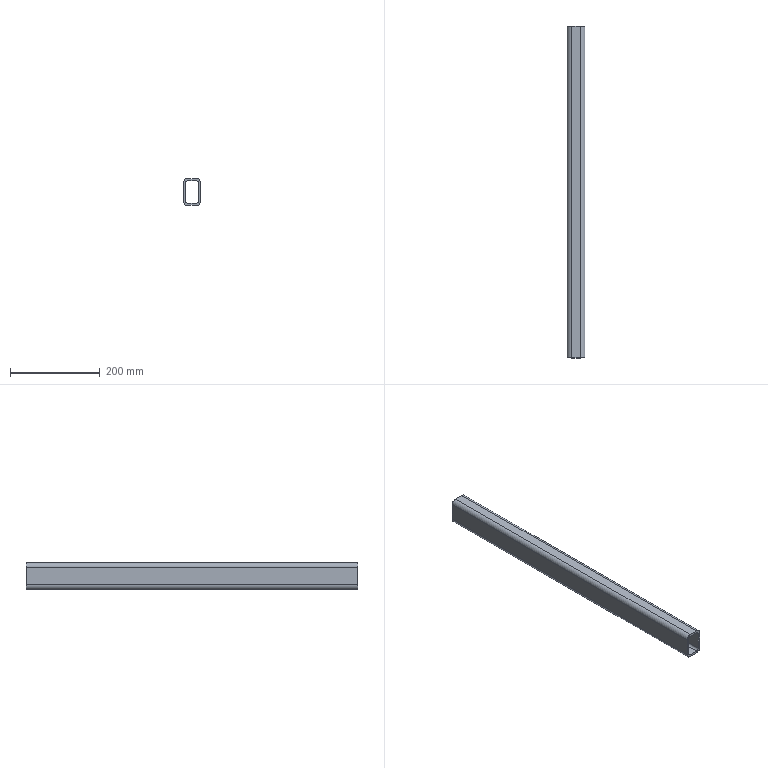Part | STEP file | HL4GD-1.30.111 base frame middle crossmember--20251212 | 1 solid | 18 faces | box 40 x 740 x 60 mm | volume 618358 mm3 | plane 10 | cylinder 8 | commonest cylinder face diameters 10 x4 20 x4
STEP:
#1=CARTESIAN_POINT('',(0.,0.,0.));
#2=DIRECTION('',(0.,0.,1.));
#3=DIRECTION('',(1.,0.,0.));
#4=AXIS2_PLACEMENT_3D('',#1,#2,#3);
#5=CARTESIAN_POINT('',(1685.,370.,410.));
#6=VERTEX_POINT('',#5);
#7=CARTESIAN_POINT('',(1680.,370.,415.));
#8=VERTEX_POINT('',#7);
#9=CARTESIAN_POINT('',(1685.,370.,415.));
#10=DIRECTION('',(0.,1.,0.));
#11=DIRECTION('',(-1.,0.,0.));
#12=AXIS2_PLACEMENT_3D('',#9,#10,#11);
#13=CIRCLE('',#12,5.);
#14=CARTESIAN_POINT('',(1685.,530.,415.));
#15=DIRECTION('',(0.,1.,0.));
#16=DIRECTION('',(-1.,0.,0.));
#17=AXIS2_PLACEMENT_3D('',#14,#15,#16);
#18=CYLINDRICAL_SURFACE('',#17,5.);
#19=CARTESIAN_POINT('',(0.,-160.));
#20=DIRECTION('',(1.,0.));
#21=VECTOR('',#20,1.);
#22=LINE('',#19,#21);
#23=(GEOMETRIC_REPRESENTATION_CONTEXT(2)PARAMETRIC_REPRESENTATION_CONTEXT()REPRESENTATION_CONTEXT('',''));
#24=DEFINITIONAL_REPRESENTATION('',(#22),#23);
#25=PCURVE('',#18,#24);
#26=CARTESIAN_POINT('',(1498.93,370.,281.07));
#27=DIRECTION('',(0.,1.,0.));
#28=DIRECTION('',(-1.,0.,0.));
#29=AXIS2_PLACEMENT_3D('',#26,#27,#28);
#30=PLANE('',#29);
#31=CARTESIAN_POINT('',(-186.07,133.93));
#32=DIRECTION('',(1.,0.));
#33=AXIS2_PLACEMENT_2D('',#31,#32);
#34=CIRCLE('',#33,5.);
#35=(GEOMETRIC_REPRESENTATION_CONTEXT(2)PARAMETRIC_REPRESENTATION_CONTEXT()REPRESENTATION_CONTEXT('',''));
#36=DEFINITIONAL_REPRESENTATION('',(#34),#35);
#37=PCURVE('',#30,#36);
#38=SURFACE_CURVE('',#13,(#25,#37),.PCURVE_S1.);
#39=EDGE_CURVE('',#6,#8,#38,.T.);
#40=ORIENTED_EDGE('',*,*,#39,.T.);
#41=CARTESIAN_POINT('',(1680.,1110.,415.));
#42=VERTEX_POINT('',#41);
#43=CARTESIAN_POINT('',(1680.,530.,415.));
#44=DIRECTION('',(0.,1.,0.));
#45=VECTOR('',#44,1.);
#46=LINE('',#43,#45);
#47=CARTESIAN_POINT('',(6.283,0.));
#48=DIRECTION('',(0.,1.));
#49=VECTOR('',#48,1.);
#50=LINE('',#47,#49);
#51=(GEOMETRIC_REPRESENTATION_CONTEXT(2)PARAMETRIC_REPRESENTATION_CONTEXT()REPRESENTATION_CONTEXT('',''));
#52=DEFINITIONAL_REPRESENTATION('',(#50),#51);
#53=PCURVE('',#18,#52);
#54=CARTESIAN_POINT('',(1680.,530.,415.));
#55=DIRECTION('',(1.,0.,0.));
#56=DIRECTION('',(0.,0.,-1.));
#57=AXIS2_PLACEMENT_3D('',#54,#55,#56);
#58=PLANE('',#57);
#59=CARTESIAN_POINT('',(0.,0.));
#60=DIRECTION('',(0.,1.));
#61=VECTOR('',#60,1.);
#62=LINE('',#59,#61);
#63=(GEOMETRIC_REPRESENTATION_CONTEXT(2)PARAMETRIC_REPRESENTATION_CONTEXT()REPRESENTATION_CONTEXT('',''));
#64=DEFINITIONAL_REPRESENTATION('',(#62),#63);
#65=PCURVE('',#58,#64);
#66=SURFACE_CURVE('',#46,(#53,#65),.PCURVE_S1.);
#67=EDGE_CURVE('',#8,#42,#66,.T.);
#68=ORIENTED_EDGE('',*,*,#67,.T.);
#69=CARTESIAN_POINT('',(1685.,1110.,410.));
#70=VERTEX_POINT('',#69);
#71=CARTESIAN_POINT('',(1685.,1110.,415.));
#72=DIRECTION('',(0.,1.,0.));
#73=DIRECTION('',(0.,0.,1.));
#74=AXIS2_PLACEMENT_3D('',#71,#72,#73);
#75=CIRCLE('',#74,5.);
#76=CARTESIAN_POINT('',(1.571,580.));
#77=DIRECTION('',(1.,0.));
#78=VECTOR('',#77,1.);
#79=LINE('',#76,#78);
#80=(GEOMETRIC_REPRESENTATION_CONTEXT(2)PARAMETRIC_REPRESENTATION_CONTEXT()REPRESENTATION_CONTEXT('',''));
#81=DEFINITIONAL_REPRESENTATION('',(#79),#80);
#82=PCURVE('',#18,#81);
#83=CARTESIAN_POINT('',(1945.,1110.,435.));
#84=DIRECTION('',(0.,1.,0.));
#85=DIRECTION('',(0.,0.,1.));
#86=AXIS2_PLACEMENT_3D('',#83,#84,#85);
#87=PLANE('',#86);
#88=CARTESIAN_POINT('',(-20.,-260.));
#89=DIRECTION('',(1.,0.));
#90=AXIS2_PLACEMENT_2D('',#88,#89);
#91=CIRCLE('',#90,5.);
#92=(GEOMETRIC_REPRESENTATION_CONTEXT(2)PARAMETRIC_REPRESENTATION_CONTEXT()REPRESENTATION_CONTEXT('',''));
#93=DEFINITIONAL_REPRESENTATION('',(#91),#92);
#94=PCURVE('',#87,#93);
#95=SURFACE_CURVE('',#75,(#82,#94),.PCURVE_S1.);
#96=EDGE_CURVE('',#70,#42,#95,.T.);
#97=ORIENTED_EDGE('',*,*,#96,.F.);
#98=CARTESIAN_POINT('',(1685.,530.,410.));
#99=DIRECTION('',(0.,1.,0.));
#100=VECTOR('',#99,1.);
#101=LINE('',#98,#100);
#102=CARTESIAN_POINT('',(4.712,0.));
#103=DIRECTION('',(0.,1.));
#104=VECTOR('',#103,1.);
#105=LINE('',#102,#104);
#106=(GEOMETRIC_REPRESENTATION_CONTEXT(2)PARAMETRIC_REPRESENTATION_CONTEXT()REPRESENTATION_CONTEXT('',''));
#107=DEFINITIONAL_REPRESENTATION('',(#105),#106);
#108=PCURVE('',#18,#107);
#109=CARTESIAN_POINT('',(1705.,530.,410.));
#110=DIRECTION('',(0.,0.,1.));
#111=DIRECTION('',(1.,0.,0.));
#112=AXIS2_PLACEMENT_3D('',#109,#110,#111);
#113=PLANE('',#112);
#114=CARTESIAN_POINT('',(-20.,0.));
#115=DIRECTION('',(0.,1.));
#116=VECTOR('',#115,1.);
#117=LINE('',#114,#116);
#118=(GEOMETRIC_REPRESENTATION_CONTEXT(2)PARAMETRIC_REPRESENTATION_CONTEXT()REPRESENTATION_CONTEXT('',''));
#119=DEFINITIONAL_REPRESENTATION('',(#117),#118);
#120=PCURVE('',#113,#119);
#121=SURFACE_CURVE('',#101,(#108,#120),.PCURVE_S1.);
#122=EDGE_CURVE('',#6,#70,#121,.T.);
#123=ORIENTED_EDGE('',*,*,#122,.F.);
#124=EDGE_LOOP('',(#40,#68,#97,#123));
#125=FACE_BOUND('',#124,.F.);
#126=ADVANCED_FACE('',(#125),#18,.F.);
#127=CARTESIAN_POINT('',(1705.,370.,410.));
#128=VERTEX_POINT('',#127);
#129=CARTESIAN_POINT('',(1705.,1110.,410.));
#130=VERTEX_POINT('',#129);
#131=CARTESIAN_POINT('',(1705.,530.,410.));
#132=DIRECTION('',(0.,1.,0.));
#133=VECTOR('',#132,1.);
#134=LINE('',#131,#133);
#135=CARTESIAN_POINT('',(0.,0.));
#136=DIRECTION('',(0.,1.));
#137=VECTOR('',#136,1.);
#138=LINE('',#135,#137);
#139=(GEOMETRIC_REPRESENTATION_CONTEXT(2)PARAMETRIC_REPRESENTATION_CONTEXT()REPRESENTATION_CONTEXT('',''));
#140=DEFINITIONAL_REPRESENTATION('',(#138),#139);
#141=PCURVE('',#113,#140);
#142=CARTESIAN_POINT('',(1705.,530.,415.));
#143=DIRECTION('',(0.,1.,0.));
#144=DIRECTION('',(-1.,0.,0.));
#145=AXIS2_PLACEMENT_3D('',#142,#143,#144);
#146=CYLINDRICAL_SURFACE('',#145,5.);
#147=CARTESIAN_POINT('',(4.712,0.));
#148=DIRECTION('',(0.,1.));
#149=VECTOR('',#148,1.);
#150=LINE('',#147,#149);
#151=(GEOMETRIC_REPRESENTATION_CONTEXT(2)PARAMETRIC_REPRESENTATION_CONTEXT()REPRESENTATION_CONTEXT('',''));
#152=DEFINITIONAL_REPRESENTATION('',(#150),#151);
#153=PCURVE('',#146,#152);
#154=SURFACE_CURVE('',#134,(#141,#153),.PCURVE_S1.);
#155=EDGE_CURVE('',#128,#130,#154,.T.);
#156=ORIENTED_EDGE('',*,*,#155,.T.);
#157=CARTESIAN_POINT('',(1705.,1110.,410.));
#158=DIRECTION('',(-1.,0.,0.));
#159=VECTOR('',#158,1.);
#160=LINE('',#157,#159);
#161=CARTESIAN_POINT('',(0.,580.));
#162=DIRECTION('',(-1.,0.));
#163=VECTOR('',#162,1.);
#164=LINE('',#161,#163);
#165=(GEOMETRIC_REPRESENTATION_CONTEXT(2)PARAMETRIC_REPRESENTATION_CONTEXT()REPRESENTATION_CONTEXT('',''));
#166=DEFINITIONAL_REPRESENTATION('',(#164),#165);
#167=PCURVE('',#113,#166);
#168=CARTESIAN_POINT('',(-25.,-240.));
#169=DIRECTION('',(0.,-1.));
#170=VECTOR('',#169,1.);
#171=LINE('',#168,#170);
#172=(GEOMETRIC_REPRESENTATION_CONTEXT(2)PARAMETRIC_REPRESENTATION_CONTEXT()REPRESENTATION_CONTEXT('',''));
#173=DEFINITIONAL_REPRESENTATION('',(#171),#172);
#174=PCURVE('',#87,#173);
#175=SURFACE_CURVE('',#160,(#167,#174),.PCURVE_S1.);
#176=EDGE_CURVE('',#130,#70,#175,.T.);
#177=ORIENTED_EDGE('',*,*,#176,.T.);
#178=ORIENTED_EDGE('',*,*,#122,.F.);
#179=CARTESIAN_POINT('',(1705.,370.,410.));
#180=DIRECTION('',(1.,0.,0.));
#181=VECTOR('',#180,1.);
#182=LINE('',#179,#181);
#183=CARTESIAN_POINT('',(0.,-160.));
#184=DIRECTION('',(1.,0.));
#185=VECTOR('',#184,1.);
#186=LINE('',#183,#185);
#187=(GEOMETRIC_REPRESENTATION_CONTEXT(2)PARAMETRIC_REPRESENTATION_CONTEXT()REPRESENTATION_CONTEXT('',''));
#188=DEFINITIONAL_REPRESENTATION('',(#186),#187);
#189=PCURVE('',#113,#188);
#190=CARTESIAN_POINT('',(-206.07,128.93));
#191=DIRECTION('',(-1.,0.));
#192=VECTOR('',#191,1.);
#193=LINE('',#190,#192);
#194=(GEOMETRIC_REPRESENTATION_CONTEXT(2)PARAMETRIC_REPRESENTATION_CONTEXT()REPRESENTATION_CONTEXT('',''));
#195=DEFINITIONAL_REPRESENTATION('',(#193),#194);
#196=PCURVE('',#30,#195);
#197=SURFACE_CURVE('',#182,(#189,#196),.PCURVE_S1.);
#198=EDGE_CURVE('',#6,#128,#197,.T.);
#199=ORIENTED_EDGE('',*,*,#198,.T.);
#200=EDGE_LOOP('',(#156,#177,#178,#199));
#201=FACE_BOUND('',#200,.T.);
#202=ADVANCED_FACE('',(#201),#113,.T.);
#203=CARTESIAN_POINT('',(1710.,370.,415.));
#204=VERTEX_POINT('',#203);
#205=CARTESIAN_POINT('',(1705.,370.,415.));
#206=DIRECTION('',(0.,-1.,0.));
#207=DIRECTION('',(-1.,0.,0.));
#208=AXIS2_PLACEMENT_3D('',#205,#206,#207);
#209=CIRCLE('',#208,5.);
#210=CARTESIAN_POINT('',(6.283,-160.));
#211=DIRECTION('',(-1.,0.));
#212=VECTOR('',#211,1.);
#213=LINE('',#210,#212);
#214=(GEOMETRIC_REPRESENTATION_CONTEXT(2)PARAMETRIC_REPRESENTATION_CONTEXT()REPRESENTATION_CONTEXT('',''));
#215=DEFINITIONAL_REPRESENTATION('',(#213),#214);
#216=PCURVE('',#146,#215);
#217=CARTESIAN_POINT('',(-201.07,133.93));
#218=CARTESIAN_POINT('',(-201.07,125.27));
#219=CARTESIAN_POINT('',(-208.57,129.6));
#220=CARTESIAN_POINT('',(-216.07,133.93));
#221=CARTESIAN_POINT('',(-208.57,138.261));
#222=CARTESIAN_POINT('',(-201.07,142.591));
#223=CARTESIAN_POINT('',(-201.07,133.93));
#224=(BOUNDED_CURVE()B_SPLINE_CURVE(2,(#217,#218,#219,#220,#221,#222,#223),.UNSPECIFIED.,.T.,.F.)B_SPLINE_CURVE_WITH_KNOTS((1,2,2,2,2,1),(-2.094,0.,2.094,4.189,6.283,8.378),.UNSPECIFIED.)CURVE()GEOMETRIC_REPRESENTATION_ITEM()RATIONAL_B_SPLINE_CURVE((1.,0.5,1.,0.5,1.,0.5,1.))REPRESENTATION_ITEM(''));
#225=(GEOMETRIC_REPRESENTATION_CONTEXT(2)PARAMETRIC_REPRESENTATION_CONTEXT()REPRESENTATION_CONTEXT('',''));
#226=DEFINITIONAL_REPRESENTATION('',(#224),#225);
#227=PCURVE('',#30,#226);
#228=SURFACE_CURVE('',#209,(#216,#227),.PCURVE_S1.);
#229=EDGE_CURVE('',#128,#204,#228,.T.);
#230=ORIENTED_EDGE('',*,*,#229,.F.);
#231=ORIENTED_EDGE('',*,*,#155,.T.);
#232=CARTESIAN_POINT('',(1710.,1110.,415.));
#233=VERTEX_POINT('',#232);
#234=CARTESIAN_POINT('',(1705.,1110.,415.));
#235=DIRECTION('',(0.,1.,0.));
#236=DIRECTION('',(0.,0.,1.));
#237=AXIS2_PLACEMENT_3D('',#234,#235,#236);
#238=CIRCLE('',#237,5.);
#239=CARTESIAN_POINT('',(1.571,580.));
#240=DIRECTION('',(1.,0.));
#241=VECTOR('',#240,1.);
#242=LINE('',#239,#241);
#243=(GEOMETRIC_REPRESENTATION_CONTEXT(2)PARAMETRIC_REPRESENTATION_CONTEXT()REPRESENTATION_CONTEXT('',''));
#244=DEFINITIONAL_REPRESENTATION('',(#242),#243);
#245=PCURVE('',#146,#244);
#246=CARTESIAN_POINT('',(-20.,-240.));
#247=DIRECTION('',(1.,0.));
#248=AXIS2_PLACEMENT_2D('',#246,#247);
#249=CIRCLE('',#248,5.);
#250=(GEOMETRIC_REPRESENTATION_CONTEXT(2)PARAMETRIC_REPRESENTATION_CONTEXT()REPRESENTATION_CONTEXT('',''));
#251=DEFINITIONAL_REPRESENTATION('',(#249),#250);
#252=PCURVE('',#87,#251);
#253=SURFACE_CURVE('',#238,(#245,#252),.PCURVE_S1.);
#254=EDGE_CURVE('',#233,#130,#253,.T.);
#255=ORIENTED_EDGE('',*,*,#254,.F.);
#256=CARTESIAN_POINT('',(1710.,530.,415.));
#257=DIRECTION('',(0.,1.,0.));
#258=VECTOR('',#257,1.);
#259=LINE('',#256,#258);
#260=CARTESIAN_POINT('',(3.142,0.));
#261=DIRECTION('',(0.,1.));
#262=VECTOR('',#261,1.);
#263=LINE('',#260,#262);
#264=(GEOMETRIC_REPRESENTATION_CONTEXT(2)PARAMETRIC_REPRESENTATION_CONTEXT()REPRESENTATION_CONTEXT('',''));
#265=DEFINITIONAL_REPRESENTATION('',(#263),#264);
#266=PCURVE('',#146,#265);
#267=CARTESIAN_POINT('',(1710.,530.,455.));
#268=DIRECTION('',(-1.,0.,0.));
#269=DIRECTION('',(0.,0.,1.));
#270=AXIS2_PLACEMENT_3D('',#267,#268,#269);
#271=PLANE('',#270);
#272=CARTESIAN_POINT('',(-40.,0.));
#273=DIRECTION('',(0.,1.));
#274=VECTOR('',#273,1.);
#275=LINE('',#272,#274);
#276=(GEOMETRIC_REPRESENTATION_CONTEXT(2)PARAMETRIC_REPRESENTATION_CONTEXT()REPRESENTATION_CONTEXT('',''));
#277=DEFINITIONAL_REPRESENTATION('',(#275),#276);
#278=PCURVE('',#271,#277);
#279=SURFACE_CURVE('',#259,(#266,#278),.PCURVE_S1.);
#280=EDGE_CURVE('',#204,#233,#279,.T.);
#281=ORIENTED_EDGE('',*,*,#280,.F.);
#282=EDGE_LOOP('',(#230,#231,#255,#281));
#283=FACE_BOUND('',#282,.F.);
#284=ADVANCED_FACE('',(#283),#146,.F.);
#285=CARTESIAN_POINT('',(1710.,370.,455.));
#286=VERTEX_POINT('',#285);
#287=CARTESIAN_POINT('',(1710.,1110.,455.));
#288=VERTEX_POINT('',#287);
#289=CARTESIAN_POINT('',(1710.,530.,455.));
#290=DIRECTION('',(0.,1.,0.));
#291=VECTOR('',#290,1.);
#292=LINE('',#289,#291);
#293=CARTESIAN_POINT('',(0.,0.));
#294=DIRECTION('',(0.,1.));
#295=VECTOR('',#294,1.);
#296=LINE('',#293,#295);
#297=(GEOMETRIC_REPRESENTATION_CONTEXT(2)PARAMETRIC_REPRESENTATION_CONTEXT()REPRESENTATION_CONTEXT('',''));
#298=DEFINITIONAL_REPRESENTATION('',(#296),#297);
#299=PCURVE('',#271,#298);
#300=CARTESIAN_POINT('',(1705.,530.,455.));
#301=DIRECTION('',(0.,1.,0.));
#302=DIRECTION('',(-1.,0.,0.));
#303=AXIS2_PLACEMENT_3D('',#300,#301,#302);
#304=CYLINDRICAL_SURFACE('',#303,5.);
#305=CARTESIAN_POINT('',(3.142,0.));
#306=DIRECTION('',(0.,1.));
#307=VECTOR('',#306,1.);
#308=LINE('',#305,#307);
#309=(GEOMETRIC_REPRESENTATION_CONTEXT(2)PARAMETRIC_REPRESENTATION_CONTEXT()REPRESENTATION_CONTEXT('',''));
#310=DEFINITIONAL_REPRESENTATION('',(#308),#309);
#311=PCURVE('',#304,#310);
#312=SURFACE_CURVE('',#292,(#299,#311),.PCURVE_S1.);
#313=EDGE_CURVE('',#286,#288,#312,.T.);
#314=ORIENTED_EDGE('',*,*,#313,.T.);
#315=CARTESIAN_POINT('',(1710.,1110.,455.));
#316=DIRECTION('',(0.,0.,-1.));
#317=VECTOR('',#316,1.);
#318=LINE('',#315,#317);
#319=CARTESIAN_POINT('',(0.,580.));
#320=DIRECTION('',(-1.,0.));
#321=VECTOR('',#320,1.);
#322=LINE('',#319,#321);
#323=(GEOMETRIC_REPRESENTATION_CONTEXT(2)PARAMETRIC_REPRESENTATION_CONTEXT()REPRESENTATION_CONTEXT('',''));
#324=DEFINITIONAL_REPRESENTATION('',(#322),#323);
#325=PCURVE('',#271,#324);
#326=CARTESIAN_POINT('',(20.,-235.));
#327=DIRECTION('',(-1.,0.));
#328=VECTOR('',#327,1.);
#329=LINE('',#326,#328);
#330=(GEOMETRIC_REPRESENTATION_CONTEXT(2)PARAMETRIC_REPRESENTATION_CONTEXT()REPRESENTATION_CONTEXT('',''));
#331=DEFINITIONAL_REPRESENTATION('',(#329),#330);
#332=PCURVE('',#87,#331);
#333=SURFACE_CURVE('',#318,(#325,#332),.PCURVE_S1.);
#334=EDGE_CURVE('',#288,#233,#333,.T.);
#335=ORIENTED_EDGE('',*,*,#334,.T.);
#336=ORIENTED_EDGE('',*,*,#280,.F.);
#337=CARTESIAN_POINT('',(1710.,370.,455.));
#338=DIRECTION('',(0.,0.,-1.));
#339=VECTOR('',#338,1.);
#340=LINE('',#337,#339);
#341=CARTESIAN_POINT('',(0.,-160.));
#342=DIRECTION('',(-1.,0.));
#343=VECTOR('',#342,1.);
#344=LINE('',#341,#343);
#345=(GEOMETRIC_REPRESENTATION_CONTEXT(2)PARAMETRIC_REPRESENTATION_CONTEXT()REPRESENTATION_CONTEXT('',''));
#346=DEFINITIONAL_REPRESENTATION('',(#344),#345);
#347=PCURVE('',#271,#346);
#348=CARTESIAN_POINT('',(-211.07,173.93));
#349=DIRECTION('',(0.,-1.));
#350=VECTOR('',#349,1.);
#351=LINE('',#348,#350);
#352=(GEOMETRIC_REPRESENTATION_CONTEXT(2)PARAMETRIC_REPRESENTATION_CONTEXT()REPRESENTATION_CONTEXT('',''));
#353=DEFINITIONAL_REPRESENTATION('',(#351),#352);
#354=PCURVE('',#30,#353);
#355=SURFACE_CURVE('',#340,(#347,#354),.PCURVE_S1.);
#356=EDGE_CURVE('',#286,#204,#355,.T.);
#357=ORIENTED_EDGE('',*,*,#356,.F.);
#358=EDGE_LOOP('',(#314,#335,#336,#357));
#359=FACE_BOUND('',#358,.T.);
#360=ADVANCED_FACE('',(#359),#271,.T.);
#361=CARTESIAN_POINT('',(1705.,370.,460.));
#362=VERTEX_POINT('',#361);
#363=CARTESIAN_POINT('',(1705.,370.,455.));
#364=DIRECTION('',(0.,1.,0.));
#365=DIRECTION('',(-1.,0.,0.));
#366=AXIS2_PLACEMENT_3D('',#363,#364,#365);
#367=CIRCLE('',#366,5.);
#368=CARTESIAN_POINT('',(0.,-160.));
#369=DIRECTION('',(1.,0.));
#370=VECTOR('',#369,1.);
#371=LINE('',#368,#370);
#372=(GEOMETRIC_REPRESENTATION_CONTEXT(2)PARAMETRIC_REPRESENTATION_CONTEXT()REPRESENTATION_CONTEXT('',''));
#373=DEFINITIONAL_REPRESENTATION('',(#371),#372);
#374=PCURVE('',#304,#373);
#375=CARTESIAN_POINT('',(-206.07,173.93));
#376=DIRECTION('',(1.,0.));
#377=AXIS2_PLACEMENT_2D('',#375,#376);
#378=CIRCLE('',#377,5.);
#379=(GEOMETRIC_REPRESENTATION_CONTEXT(2)PARAMETRIC_REPRESENTATION_CONTEXT()REPRESENTATION_CONTEXT('',''));
#380=DEFINITIONAL_REPRESENTATION('',(#378),#379);
#381=PCURVE('',#30,#380);
#382=SURFACE_CURVE('',#367,(#374,#381),.PCURVE_S1.);
#383=EDGE_CURVE('',#362,#286,#382,.T.);
#384=ORIENTED_EDGE('',*,*,#383,.T.);
#385=ORIENTED_EDGE('',*,*,#313,.T.);
#386=CARTESIAN_POINT('',(1705.,1110.,460.));
#387=VERTEX_POINT('',#386);
#388=CARTESIAN_POINT('',(1705.,1110.,455.));
#389=DIRECTION('',(0.,1.,0.));
#390=DIRECTION('',(0.,0.,1.));
#391=AXIS2_PLACEMENT_3D('',#388,#389,#390);
#392=CIRCLE('',#391,5.);
#393=CARTESIAN_POINT('',(1.571,580.));
#394=DIRECTION('',(1.,0.));
#395=VECTOR('',#394,1.);
#396=LINE('',#393,#395);
#397=(GEOMETRIC_REPRESENTATION_CONTEXT(2)PARAMETRIC_REPRESENTATION_CONTEXT()REPRESENTATION_CONTEXT('',''));
#398=DEFINITIONAL_REPRESENTATION('',(#396),#397);
#399=PCURVE('',#304,#398);
#400=CARTESIAN_POINT('',(20.,-240.));
#401=DIRECTION('',(1.,0.));
#402=AXIS2_PLACEMENT_2D('',#400,#401);
#403=CIRCLE('',#402,5.);
#404=(GEOMETRIC_REPRESENTATION_CONTEXT(2)PARAMETRIC_REPRESENTATION_CONTEXT()REPRESENTATION_CONTEXT('',''));
#405=DEFINITIONAL_REPRESENTATION('',(#403),#404);
#406=PCURVE('',#87,#405);
#407=SURFACE_CURVE('',#392,(#399,#406),.PCURVE_S1.);
#408=EDGE_CURVE('',#387,#288,#407,.T.);
#409=ORIENTED_EDGE('',*,*,#408,.F.);
#410=CARTESIAN_POINT('',(1705.,530.,460.));
#411=DIRECTION('',(0.,1.,0.));
#412=VECTOR('',#411,1.);
#413=LINE('',#410,#412);
#414=CARTESIAN_POINT('',(1.571,0.));
#415=DIRECTION('',(0.,1.));
#416=VECTOR('',#415,1.);
#417=LINE('',#414,#416);
#418=(GEOMETRIC_REPRESENTATION_CONTEXT(2)PARAMETRIC_REPRESENTATION_CONTEXT()REPRESENTATION_CONTEXT('',''));
#419=DEFINITIONAL_REPRESENTATION('',(#417),#418);
#420=PCURVE('',#304,#419);
#421=CARTESIAN_POINT('',(1685.,530.,460.));
#422=DIRECTION('',(0.,0.,-1.));
#423=DIRECTION('',(-1.,0.,0.));
#424=AXIS2_PLACEMENT_3D('',#421,#422,#423);
#425=PLANE('',#424);
#426=CARTESIAN_POINT('',(-20.,0.));
#427=DIRECTION('',(0.,1.));
#428=VECTOR('',#427,1.);
#429=LINE('',#426,#428);
#430=(GEOMETRIC_REPRESENTATION_CONTEXT(2)PARAMETRIC_REPRESENTATION_CONTEXT()REPRESENTATION_CONTEXT('',''));
#431=DEFINITIONAL_REPRESENTATION('',(#429),#430);
#432=PCURVE('',#425,#431);
#433=SURFACE_CURVE('',#413,(#420,#432),.PCURVE_S1.);
#434=EDGE_CURVE('',#362,#387,#433,.T.);
#435=ORIENTED_EDGE('',*,*,#434,.F.);
#436=EDGE_LOOP('',(#384,#385,#409,#435));
#437=FACE_BOUND('',#436,.F.);
#438=ADVANCED_FACE('',(#437),#304,.F.);
#439=CARTESIAN_POINT('',(1685.,370.,460.));
#440=VERTEX_POINT('',#439);
#441=CARTESIAN_POINT('',(1685.,1110.,460.));
#442=VERTEX_POINT('',#441);
#443=CARTESIAN_POINT('',(1685.,530.,460.));
#444=DIRECTION('',(0.,1.,0.));
#445=VECTOR('',#444,1.);
#446=LINE('',#443,#445);
#447=CARTESIAN_POINT('',(0.,0.));
#448=DIRECTION('',(0.,1.));
#449=VECTOR('',#448,1.);
#450=LINE('',#447,#449);
#451=(GEOMETRIC_REPRESENTATION_CONTEXT(2)PARAMETRIC_REPRESENTATION_CONTEXT()REPRESENTATION_CONTEXT('',''));
#452=DEFINITIONAL_REPRESENTATION('',(#450),#451);
#453=PCURVE('',#425,#452);
#454=CARTESIAN_POINT('',(1685.,530.,455.));
#455=DIRECTION('',(0.,1.,0.));
#456=DIRECTION('',(-1.,0.,0.));
#457=AXIS2_PLACEMENT_3D('',#454,#455,#456);
#458=CYLINDRICAL_SURFACE('',#457,5.);
#459=CARTESIAN_POINT('',(1.571,0.));
#460=DIRECTION('',(0.,1.));
#461=VECTOR('',#460,1.);
#462=LINE('',#459,#461);
#463=(GEOMETRIC_REPRESENTATION_CONTEXT(2)PARAMETRIC_REPRESENTATION_CONTEXT()REPRESENTATION_CONTEXT('',''));
#464=DEFINITIONAL_REPRESENTATION('',(#462),#463);
#465=PCURVE('',#458,#464);
#466=SURFACE_CURVE('',#446,(#453,#465),.PCURVE_S1.);
#467=EDGE_CURVE('',#440,#442,#466,.T.);
#468=ORIENTED_EDGE('',*,*,#467,.T.);
#469=CARTESIAN_POINT('',(1685.,1110.,460.));
#470=DIRECTION('',(1.,0.,0.));
#471=VECTOR('',#470,1.);
#472=LINE('',#469,#471);
#473=CARTESIAN_POINT('',(0.,580.));
#474=DIRECTION('',(-1.,0.));
#475=VECTOR('',#474,1.);
#476=LINE('',#473,#475);
#477=(GEOMETRIC_REPRESENTATION_CONTEXT(2)PARAMETRIC_REPRESENTATION_CONTEXT()REPRESENTATION_CONTEXT('',''));
#478=DEFINITIONAL_REPRESENTATION('',(#476),#477);
#479=PCURVE('',#425,#478);
#480=CARTESIAN_POINT('',(25.,-260.));
#481=DIRECTION('',(0.,1.));
#482=VECTOR('',#481,1.);
#483=LINE('',#480,#482);
#484=(GEOMETRIC_REPRESENTATION_CONTEXT(2)PARAMETRIC_REPRESENTATION_CONTEXT()REPRESENTATION_CONTEXT('',''));
#485=DEFINITIONAL_REPRESENTATION('',(#483),#484);
#486=PCURVE('',#87,#485);
#487=SURFACE_CURVE('',#472,(#479,#486),.PCURVE_S1.);
#488=EDGE_CURVE('',#442,#387,#487,.T.);
#489=ORIENTED_EDGE('',*,*,#488,.T.);
#490=ORIENTED_EDGE('',*,*,#434,.F.);
#491=CARTESIAN_POINT('',(1685.,370.,460.));
#492=DIRECTION('',(1.,0.,0.));
#493=VECTOR('',#492,1.);
#494=LINE('',#491,#493);
#495=CARTESIAN_POINT('',(0.,-160.));
#496=DIRECTION('',(-1.,0.));
#497=VECTOR('',#496,1.);
#498=LINE('',#495,#497);
#499=(GEOMETRIC_REPRESENTATION_CONTEXT(2)PARAMETRIC_REPRESENTATION_CONTEXT()REPRESENTATION_CONTEXT('',''));
#500=DEFINITIONAL_REPRESENTATION('',(#498),#499);
#501=PCURVE('',#425,#500);
#502=CARTESIAN_POINT('',(-186.07,178.93));
#503=DIRECTION('',(-1.,0.));
#504=VECTOR('',#503,1.);
#505=LINE('',#502,#504);
#506=(GEOMETRIC_REPRESENTATION_CONTEXT(2)PARAMETRIC_REPRESENTATION_CONTEXT()REPRESENTATION_CONTEXT('',''));
#507=DEFINITIONAL_REPRESENTATION('',(#505),#506);
#508=PCURVE('',#30,#507);
#509=SURFACE_CURVE('',#494,(#501,#508),.PCURVE_S1.);
#510=EDGE_CURVE('',#440,#362,#509,.T.);
#511=ORIENTED_EDGE('',*,*,#510,.F.);
#512=EDGE_LOOP('',(#468,#489,#490,#511));
#513=FACE_BOUND('',#512,.T.);
#514=ADVANCED_FACE('',(#513),#425,.T.);
#515=CARTESIAN_POINT('',(1680.,370.,455.));
#516=VERTEX_POINT('',#515);
#517=CARTESIAN_POINT('',(1685.,370.,455.));
#518=DIRECTION('',(0.,-1.,0.));
#519=DIRECTION('',(-1.,0.,0.));
#520=AXIS2_PLACEMENT_3D('',#517,#518,#519);
#521=CIRCLE('',#520,5.);
#522=CARTESIAN_POINT('',(6.283,-160.));
#523=DIRECTION('',(-1.,0.));
#524=VECTOR('',#523,1.);
#525=LINE('',#522,#524);
#526=(GEOMETRIC_REPRESENTATION_CONTEXT(2)PARAMETRIC_REPRESENTATION_CONTEXT()REPRESENTATION_CONTEXT('',''));
#527=DEFINITIONAL_REPRESENTATION('',(#525),#526);
#528=PCURVE('',#458,#527);
#529=CARTESIAN_POINT('',(-181.07,173.93));
#530=CARTESIAN_POINT('',(-181.07,165.27));
#531=CARTESIAN_POINT('',(-188.57,169.6));
#532=CARTESIAN_POINT('',(-196.07,173.93));
#533=CARTESIAN_POINT('',(-188.57,178.261));
#534=CARTESIAN_POINT('',(-181.07,182.591));
#535=CARTESIAN_POINT('',(-181.07,173.93));
#536=(BOUNDED_CURVE()B_SPLINE_CURVE(2,(#529,#530,#531,#532,#533,#534,#535),.UNSPECIFIED.,.T.,.F.)B_SPLINE_CURVE_WITH_KNOTS((1,2,2,2,2,1),(-2.094,0.,2.094,4.189,6.283,8.378),.UNSPECIFIED.)CURVE()GEOMETRIC_REPRESENTATION_ITEM()RATIONAL_B_SPLINE_CURVE((1.,0.5,1.,0.5,1.,0.5,1.))REPRESENTATION_ITEM(''));
#537=(GEOMETRIC_REPRESENTATION_CONTEXT(2)PARAMETRIC_REPRESENTATION_CONTEXT()REPRESENTATION_CONTEXT('',''));
#538=DEFINITIONAL_REPRESENTATION('',(#536),#537);
#539=PCURVE('',#30,#538);
#540=SURFACE_CURVE('',#521,(#528,#539),.PCURVE_S1.);
#541=EDGE_CURVE('',#440,#516,#540,.T.);
#542=ORIENTED_EDGE('',*,*,#541,.F.);
#543=ORIENTED_EDGE('',*,*,#467,.T.);
#544=CARTESIAN_POINT('',(1680.,1110.,455.));
#545=VERTEX_POINT('',#544);
#546=CARTESIAN_POINT('',(1685.,1110.,455.));
#547=DIRECTION('',(0.,1.,0.));
#548=DIRECTION('',(0.,0.,1.));
#549=AXIS2_PLACEMENT_3D('',#546,#547,#548);
#550=CIRCLE('',#549,5.);
#551=CARTESIAN_POINT('',(-4.712,580.));
#552=DIRECTION('',(1.,0.));
#553=VECTOR('',#552,1.);
#554=LINE('',#551,#553);
#555=(GEOMETRIC_REPRESENTATION_CONTEXT(2)PARAMETRIC_REPRESENTATION_CONTEXT()REPRESENTATION_CONTEXT('',''));
#556=DEFINITIONAL_REPRESENTATION('',(#554),#555);
#557=PCURVE('',#458,#556);
#558=CARTESIAN_POINT('',(20.,-260.));
#559=DIRECTION('',(1.,0.));
#560=AXIS2_PLACEMENT_2D('',#558,#559);
#561=CIRCLE('',#560,5.);
#562=(GEOMETRIC_REPRESENTATION_CONTEXT(2)PARAMETRIC_REPRESENTATION_CONTEXT()REPRESENTATION_CONTEXT('',''));
#563=DEFINITIONAL_REPRESENTATION('',(#561),#562);
#564=PCURVE('',#87,#563);
#565=SURFACE_CURVE('',#550,(#557,#564),.PCURVE_S1.);
#566=EDGE_CURVE('',#545,#442,#565,.T.);
#567=ORIENTED_EDGE('',*,*,#566,.F.);
#568=CARTESIAN_POINT('',(1680.,530.,455.));
#569=DIRECTION('',(0.,1.,0.));
#570=VECTOR('',#569,1.);
#571=LINE('',#568,#570);
#572=CARTESIAN_POINT('',(0.,0.));
#573=DIRECTION('',(0.,1.));
#574=VECTOR('',#573,1.);
#575=LINE('',#572,#574);
#576=(GEOMETRIC_REPRESENTATION_CONTEXT(2)PARAMETRIC_REPRESENTATION_CONTEXT()REPRESENTATION_CONTEXT('',''));
#577=DEFINITIONAL_REPRESENTATION('',(#575),#576);
#578=PCURVE('',#458,#577);
#579=CARTESIAN_POINT('',(-40.,0.));
#580=DIRECTION('',(0.,1.));
#581=VECTOR('',#580,1.);
#582=LINE('',#579,#581);
#583=(GEOMETRIC_REPRESENTATION_CONTEXT(2)PARAMETRIC_REPRESENTATION_CONTEXT()REPRESENTATION_CONTEXT('',''));
#584=DEFINITIONAL_REPRESENTATION('',(#582),#583);
#585=PCURVE('',#58,#584);
#586=SURFACE_CURVE('',#571,(#578,#585),.PCURVE_S1.);
#587=EDGE_CURVE('',#516,#545,#586,.T.);
#588=ORIENTED_EDGE('',*,*,#587,.F.);
#589=EDGE_LOOP('',(#542,#543,#567,#588));
#590=FACE_BOUND('',#589,.F.);
#591=ADVANCED_FACE('',(#590),#458,.F.);
#592=CARTESIAN_POINT('',(1715.,370.,415.));
#593=VERTEX_POINT('',#592);
#594=CARTESIAN_POINT('',(1715.,1110.,415.));
#595=VERTEX_POINT('',#594);
#596=CARTESIAN_POINT('',(1715.,530.,415.));
#597=DIRECTION('',(0.,1.,0.));
#598=VECTOR('',#597,1.);
#599=LINE('',#596,#598);
#600=CARTESIAN_POINT('',(1715.,530.,455.));
#601=DIRECTION('',(-1.,0.,0.));
#602=DIRECTION('',(0.,0.,1.));
#603=AXIS2_PLACEMENT_3D('',#600,#601,#602);
#604=PLANE('',#603);
#605=CARTESIAN_POINT('',(-40.,0.));
#606=DIRECTION('',(0.,1.));
#607=VECTOR('',#606,1.);
#608=LINE('',#605,#607);
#609=(GEOMETRIC_REPRESENTATION_CONTEXT(2)PARAMETRIC_REPRESENTATION_CONTEXT()REPRESENTATION_CONTEXT('',''));
#610=DEFINITIONAL_REPRESENTATION('',(#608),#609);
#611=PCURVE('',#604,#610);
#612=CARTESIAN_POINT('',(1705.,530.,415.));
#613=DIRECTION('',(0.,1.,0.));
#614=DIRECTION('',(-1.,0.,0.));
#615=AXIS2_PLACEMENT_3D('',#612,#613,#614);
#616=CYLINDRICAL_SURFACE('',#615,10.);
#617=CARTESIAN_POINT('',(3.142,0.));
#618=DIRECTION('',(0.,1.));
#619=VECTOR('',#618,1.);
#620=LINE('',#617,#619);
#621=(GEOMETRIC_REPRESENTATION_CONTEXT(2)PARAMETRIC_REPRESENTATION_CONTEXT()REPRESENTATION_CONTEXT('',''));
#622=DEFINITIONAL_REPRESENTATION('',(#620),#621);
#623=PCURVE('',#616,#622);
#624=SURFACE_CURVE('',#599,(#611,#623),.PCURVE_S1.);
#625=EDGE_CURVE('',#593,#595,#624,.T.);
#626=ORIENTED_EDGE('',*,*,#625,.T.);
#627=CARTESIAN_POINT('',(1715.,1110.,455.));
#628=VERTEX_POINT('',#627);
#629=CARTESIAN_POINT('',(1715.,1110.,455.));
#630=DIRECTION('',(0.,0.,1.));
#631=VECTOR('',#630,1.);
#632=LINE('',#629,#631);
#633=CARTESIAN_POINT('',(0.,580.));
#634=DIRECTION('',(1.,0.));
#635=VECTOR('',#634,1.);
#636=LINE('',#633,#635);
#637=(GEOMETRIC_REPRESENTATION_CONTEXT(2)PARAMETRIC_REPRESENTATION_CONTEXT()REPRESENTATION_CONTEXT('',''));
#638=DEFINITIONAL_REPRESENTATION('',(#636),#637);
#639=PCURVE('',#604,#638);
#640=CARTESIAN_POINT('',(20.,-230.));
#641=DIRECTION('',(1.,0.));
#642=VECTOR('',#641,1.);
#643=LINE('',#640,#642);
#644=(GEOMETRIC_REPRESENTATION_CONTEXT(2)PARAMETRIC_REPRESENTATION_CONTEXT()REPRESENTATION_CONTEXT('',''));
#645=DEFINITIONAL_REPRESENTATION('',(#643),#644);
#646=PCURVE('',#87,#645);
#647=SURFACE_CURVE('',#632,(#639,#646),.PCURVE_S1.);
#648=EDGE_CURVE('',#595,#628,#647,.T.);
#649=ORIENTED_EDGE('',*,*,#648,.T.);
#650=CARTESIAN_POINT('',(1715.,370.,455.));
#651=VERTEX_POINT('',#650);
#652=CARTESIAN_POINT('',(1715.,530.,455.));
#653=DIRECTION('',(0.,1.,0.));
#654=VECTOR('',#653,1.);
#655=LINE('',#652,#654);
#656=CARTESIAN_POINT('',(0.,0.));
#657=DIRECTION('',(0.,1.));
#658=VECTOR('',#657,1.);
#659=LINE('',#656,#658);
#660=(GEOMETRIC_REPRESENTATION_CONTEXT(2)PARAMETRIC_REPRESENTATION_CONTEXT()REPRESENTATION_CONTEXT('',''));
#661=DEFINITIONAL_REPRESENTATION('',(#659),#660);
#662=PCURVE('',#604,#661);
#663=CARTESIAN_POINT('',(1705.,530.,455.));
#664=DIRECTION('',(0.,1.,0.));
#665=DIRECTION('',(-1.,0.,0.));
#666=AXIS2_PLACEMENT_3D('',#663,#664,#665);
#667=CYLINDRICAL_SURFACE('',#666,10.);
#668=CARTESIAN_POINT('',(3.142,0.));
#669=DIRECTION('',(0.,1.));
#670=VECTOR('',#669,1.);
#671=LINE('',#668,#670);
#672=(GEOMETRIC_REPRESENTATION_CONTEXT(2)PARAMETRIC_REPRESENTATION_CONTEXT()REPRESENTATION_CONTEXT('',''));
#673=DEFINITIONAL_REPRESENTATION('',(#671),#672);
#674=PCURVE('',#667,#673);
#675=SURFACE_CURVE('',#655,(#662,#674),.PCURVE_S1.);
#676=EDGE_CURVE('',#651,#628,#675,.T.);
#677=ORIENTED_EDGE('',*,*,#676,.F.);
#678=CARTESIAN_POINT('',(1715.,370.,455.));
#679=DIRECTION('',(0.,0.,1.));
#680=VECTOR('',#679,1.);
#681=LINE('',#678,#680);
#682=CARTESIAN_POINT('',(0.,-160.));
#683=DIRECTION('',(1.,0.));
#684=VECTOR('',#683,1.);
#685=LINE('',#682,#684);
#686=(GEOMETRIC_REPRESENTATION_CONTEXT(2)PARAMETRIC_REPRESENTATION_CONTEXT()REPRESENTATION_CONTEXT('',''));
#687=DEFINITIONAL_REPRESENTATION('',(#685),#686);
#688=PCURVE('',#604,#687);
#689=CARTESIAN_POINT('',(-216.07,173.93));
#690=DIRECTION('',(0.,1.));
#691=VECTOR('',#690,1.);
#692=LINE('',#689,#691);
#693=(GEOMETRIC_REPRESENTATION_CONTEXT(2)PARAMETRIC_REPRESENTATION_CONTEXT()REPRESENTATION_CONTEXT('',''));
#694=DEFINITIONAL_REPRESENTATION('',(#692),#693);
#695=PCURVE('',#30,#694);
#696=SURFACE_CURVE('',#681,(#688,#695),.PCURVE_S1.);
#697=EDGE_CURVE('',#593,#651,#696,.T.);
#698=ORIENTED_EDGE('',*,*,#697,.F.);
#699=EDGE_LOOP('',(#626,#649,#677,#698));
#700=FACE_BOUND('',#699,.T.);
#701=ADVANCED_FACE('',(#700),#604,.F.);
#702=CARTESIAN_POINT('',(1705.,370.,405.));
#703=VERTEX_POINT('',#702);
#704=CARTESIAN_POINT('',(1705.,1110.,405.));
#705=VERTEX_POINT('',#704);
#706=CARTESIAN_POINT('',(1705.,530.,405.));
#707=DIRECTION('',(0.,1.,0.));
#708=VECTOR('',#707,1.);
#709=LINE('',#706,#708);
#710=CARTESIAN_POINT('',(4.712,0.));
#711=DIRECTION('',(0.,1.));
#712=VECTOR('',#711,1.);
#713=LINE('',#710,#712);
#714=(GEOMETRIC_REPRESENTATION_CONTEXT(2)PARAMETRIC_REPRESENTATION_CONTEXT()REPRESENTATION_CONTEXT('',''));
#715=DEFINITIONAL_REPRESENTATION('',(#713),#714);
#716=PCURVE('',#616,#715);
#717=CARTESIAN_POINT('',(1705.,530.,405.));
#718=DIRECTION('',(0.,0.,1.));
#719=DIRECTION('',(1.,0.,0.));
#720=AXIS2_PLACEMENT_3D('',#717,#718,#719);
#721=PLANE('',#720);
#722=CARTESIAN_POINT('',(0.,0.));
#723=DIRECTION('',(0.,1.));
#724=VECTOR('',#723,1.);
#725=LINE('',#722,#724);
#726=(GEOMETRIC_REPRESENTATION_CONTEXT(2)PARAMETRIC_REPRESENTATION_CONTEXT()REPRESENTATION_CONTEXT('',''));
#727=DEFINITIONAL_REPRESENTATION('',(#725),#726);
#728=PCURVE('',#721,#727);
#729=SURFACE_CURVE('',#709,(#716,#728),.PCURVE_S1.);
#730=EDGE_CURVE('',#703,#705,#729,.T.);
#731=ORIENTED_EDGE('',*,*,#730,.T.);
#732=CARTESIAN_POINT('',(1705.,1110.,415.));
#733=DIRECTION('',(0.,-1.,0.));
#734=DIRECTION('',(0.,0.,1.));
#735=AXIS2_PLACEMENT_3D('',#732,#733,#734);
#736=CIRCLE('',#735,10.);
#737=CARTESIAN_POINT('',(7.854,580.));
#738=DIRECTION('',(-1.,0.));
#739=VECTOR('',#738,1.);
#740=LINE('',#737,#739);
#741=(GEOMETRIC_REPRESENTATION_CONTEXT(2)PARAMETRIC_REPRESENTATION_CONTEXT()REPRESENTATION_CONTEXT('',''));
#742=DEFINITIONAL_REPRESENTATION('',(#740),#741);
#743=PCURVE('',#616,#742);
#744=CARTESIAN_POINT('',(-10.,-240.));
#745=CARTESIAN_POINT('',(-10.,-257.321));
#746=CARTESIAN_POINT('',(-25.,-248.66));
#747=CARTESIAN_POINT('',(-40.,-240.));
#748=CARTESIAN_POINT('',(-25.,-231.34));
#749=CARTESIAN_POINT('',(-10.,-222.679));
#750=CARTESIAN_POINT('',(-10.,-240.));
#751=(BOUNDED_CURVE()B_SPLINE_CURVE(2,(#744,#745,#746,#747,#748,#749,#750),.UNSPECIFIED.,.T.,.F.)B_SPLINE_CURVE_WITH_KNOTS((1,2,2,2,2,1),(-2.094,0.,2.094,4.189,6.283,8.378),.UNSPECIFIED.)CURVE()GEOMETRIC_REPRESENTATION_ITEM()RATIONAL_B_SPLINE_CURVE((1.,0.5,1.,0.5,1.,0.5,1.))REPRESENTATION_ITEM(''));
#752=(GEOMETRIC_REPRESENTATION_CONTEXT(2)PARAMETRIC_REPRESENTATION_CONTEXT()REPRESENTATION_CONTEXT('',''));
#753=DEFINITIONAL_REPRESENTATION('',(#751),#752);
#754=PCURVE('',#87,#753);
#755=SURFACE_CURVE('',#736,(#743,#754),.PCURVE_S1.);
#756=EDGE_CURVE('',#705,#595,#755,.T.);
#757=ORIENTED_EDGE('',*,*,#756,.T.);
#758=ORIENTED_EDGE('',*,*,#625,.F.);
#759=CARTESIAN_POINT('',(1705.,370.,415.));
#760=DIRECTION('',(0.,-1.,0.));
#761=DIRECTION('',(-1.,0.,0.));
#762=AXIS2_PLACEMENT_3D('',#759,#760,#761);
#763=CIRCLE('',#762,10.);
#764=CARTESIAN_POINT('',(6.283,-160.));
#765=DIRECTION('',(-1.,0.));
#766=VECTOR('',#765,1.);
#767=LINE('',#764,#766);
#768=(GEOMETRIC_REPRESENTATION_CONTEXT(2)PARAMETRIC_REPRESENTATION_CONTEXT()REPRESENTATION_CONTEXT('',''));
#769=DEFINITIONAL_REPRESENTATION('',(#767),#768);
#770=PCURVE('',#616,#769);
#771=CARTESIAN_POINT('',(-196.07,133.93));
#772=CARTESIAN_POINT('',(-196.07,116.61));
#773=CARTESIAN_POINT('',(-211.07,125.27));
#774=CARTESIAN_POINT('',(-226.07,133.93));
#775=CARTESIAN_POINT('',(-211.07,142.591));
#776=CARTESIAN_POINT('',(-196.07,151.251));
#777=CARTESIAN_POINT('',(-196.07,133.93));
#778=(BOUNDED_CURVE()B_SPLINE_CURVE(2,(#771,#772,#773,#774,#775,#776,#777),.UNSPECIFIED.,.T.,.F.)B_SPLINE_CURVE_WITH_KNOTS((1,2,2,2,2,1),(-2.094,0.,2.094,4.189,6.283,8.378),.UNSPECIFIED.)CURVE()GEOMETRIC_REPRESENTATION_ITEM()RATIONAL_B_SPLINE_CURVE((1.,0.5,1.,0.5,1.,0.5,1.))REPRESENTATION_ITEM(''));
#779=(GEOMETRIC_REPRESENTATION_CONTEXT(2)PARAMETRIC_REPRESENTATION_CONTEXT()REPRESENTATION_CONTEXT('',''));
#780=DEFINITIONAL_REPRESENTATION('',(#778),#779);
#781=PCURVE('',#30,#780);
#782=SURFACE_CURVE('',#763,(#770,#781),.PCURVE_S1.);
#783=EDGE_CURVE('',#703,#593,#782,.T.);
#784=ORIENTED_EDGE('',*,*,#783,.F.);
#785=EDGE_LOOP('',(#731,#757,#758,#784));
#786=FACE_BOUND('',#785,.T.);
#787=ADVANCED_FACE('',(#786),#616,.T.);
#788=CARTESIAN_POINT('',(1685.,370.,405.));
#789=VERTEX_POINT('',#788);
#790=CARTESIAN_POINT('',(1685.,1110.,405.));
#791=VERTEX_POINT('',#790);
#792=CARTESIAN_POINT('',(1685.,530.,405.));
#793=DIRECTION('',(0.,1.,0.));
#794=VECTOR('',#793,1.);
#795=LINE('',#792,#794);
#796=CARTESIAN_POINT('',(-20.,0.));
#797=DIRECTION('',(0.,1.));
#798=VECTOR('',#797,1.);
#799=LINE('',#796,#798);
#800=(GEOMETRIC_REPRESENTATION_CONTEXT(2)PARAMETRIC_REPRESENTATION_CONTEXT()REPRESENTATION_CONTEXT('',''));
#801=DEFINITIONAL_REPRESENTATION('',(#799),#800);
#802=PCURVE('',#721,#801);
#803=CARTESIAN_POINT('',(1685.,530.,415.));
#804=DIRECTION('',(0.,1.,0.));
#805=DIRECTION('',(-1.,0.,0.));
#806=AXIS2_PLACEMENT_3D('',#803,#804,#805);
#807=CYLINDRICAL_SURFACE('',#806,10.);
#808=CARTESIAN_POINT('',(4.712,0.));
#809=DIRECTION('',(0.,1.));
#810=VECTOR('',#809,1.);
#811=LINE('',#808,#810);
#812=(GEOMETRIC_REPRESENTATION_CONTEXT(2)PARAMETRIC_REPRESENTATION_CONTEXT()REPRESENTATION_CONTEXT('',''));
#813=DEFINITIONAL_REPRESENTATION('',(#811),#812);
#814=PCURVE('',#807,#813);
#815=SURFACE_CURVE('',#795,(#802,#814),.PCURVE_S1.);
#816=EDGE_CURVE('',#789,#791,#815,.T.);
#817=ORIENTED_EDGE('',*,*,#816,.T.);
#818=CARTESIAN_POINT('',(1705.,1110.,405.));
#819=DIRECTION('',(1.,0.,0.));
#820=VECTOR('',#819,1.);
#821=LINE('',#818,#820);
#822=CARTESIAN_POINT('',(0.,580.));
#823=DIRECTION('',(1.,0.));
#824=VECTOR('',#823,1.);
#825=LINE('',#822,#824);
#826=(GEOMETRIC_REPRESENTATION_CONTEXT(2)PARAMETRIC_REPRESENTATION_CONTEXT()REPRESENTATION_CONTEXT('',''));
#827=DEFINITIONAL_REPRESENTATION('',(#825),#826);
#828=PCURVE('',#721,#827);
#829=CARTESIAN_POINT('',(-30.,-240.));
#830=DIRECTION('',(0.,1.));
#831=VECTOR('',#830,1.);
#832=LINE('',#829,#831);
#833=(GEOMETRIC_REPRESENTATION_CONTEXT(2)PARAMETRIC_REPRESENTATION_CONTEXT()REPRESENTATION_CONTEXT('',''));
#834=DEFINITIONAL_REPRESENTATION('',(#832),#833);
#835=PCURVE('',#87,#834);
#836=SURFACE_CURVE('',#821,(#828,#835),.PCURVE_S1.);
#837=EDGE_CURVE('',#791,#705,#836,.T.);
#838=ORIENTED_EDGE('',*,*,#837,.T.);
#839=ORIENTED_EDGE('',*,*,#730,.F.);
#840=CARTESIAN_POINT('',(1705.,370.,405.));
#841=DIRECTION('',(1.,0.,0.));
#842=VECTOR('',#841,1.);
#843=LINE('',#840,#842);
#844=CARTESIAN_POINT('',(0.,-160.));
#845=DIRECTION('',(1.,0.));
#846=VECTOR('',#845,1.);
#847=LINE('',#844,#846);
#848=(GEOMETRIC_REPRESENTATION_CONTEXT(2)PARAMETRIC_REPRESENTATION_CONTEXT()REPRESENTATION_CONTEXT('',''));
#849=DEFINITIONAL_REPRESENTATION('',(#847),#848);
#850=PCURVE('',#721,#849);
#851=CARTESIAN_POINT('',(-206.07,123.93));
#852=DIRECTION('',(-1.,0.));
#853=VECTOR('',#852,1.);
#854=LINE('',#851,#853);
#855=(GEOMETRIC_REPRESENTATION_CONTEXT(2)PARAMETRIC_REPRESENTATION_CONTEXT()REPRESENTATION_CONTEXT('',''));
#856=DEFINITIONAL_REPRESENTATION('',(#854),#855);
#857=PCURVE('',#30,#856);
#858=SURFACE_CURVE('',#843,(#850,#857),.PCURVE_S1.);
#859=EDGE_CURVE('',#789,#703,#858,.T.);
#860=ORIENTED_EDGE('',*,*,#859,.F.);
#861=EDGE_LOOP('',(#817,#838,#839,#860));
#862=FACE_BOUND('',#861,.T.);
#863=ADVANCED_FACE('',(#862),#721,.F.);
#864=CARTESIAN_POINT('',(1675.,370.,415.));
#865=VERTEX_POINT('',#864);
#866=CARTESIAN_POINT('',(1675.,1110.,415.));
#867=VERTEX_POINT('',#866);
#868=CARTESIAN_POINT('',(1675.,530.,415.));
#869=DIRECTION('',(0.,1.,0.));
#870=VECTOR('',#869,1.);
#871=LINE('',#868,#870);
#872=CARTESIAN_POINT('',(6.283,0.));
#873=DIRECTION('',(0.,1.));
#874=VECTOR('',#873,1.);
#875=LINE('',#872,#874);
#876=(GEOMETRIC_REPRESENTATION_CONTEXT(2)PARAMETRIC_REPRESENTATION_CONTEXT()REPRESENTATION_CONTEXT('',''));
#877=DEFINITIONAL_REPRESENTATION('',(#875),#876);
#878=PCURVE('',#807,#877);
#879=CARTESIAN_POINT('',(1675.,530.,415.));
#880=DIRECTION('',(1.,0.,0.));
#881=DIRECTION('',(0.,0.,-1.));
#882=AXIS2_PLACEMENT_3D('',#879,#880,#881);
#883=PLANE('',#882);
#884=CARTESIAN_POINT('',(0.,0.));
#885=DIRECTION('',(0.,1.));
#886=VECTOR('',#885,1.);
#887=LINE('',#884,#886);
#888=(GEOMETRIC_REPRESENTATION_CONTEXT(2)PARAMETRIC_REPRESENTATION_CONTEXT()REPRESENTATION_CONTEXT('',''));
#889=DEFINITIONAL_REPRESENTATION('',(#887),#888);
#890=PCURVE('',#883,#889);
#891=SURFACE_CURVE('',#871,(#878,#890),.PCURVE_S1.);
#892=EDGE_CURVE('',#865,#867,#891,.T.);
#893=ORIENTED_EDGE('',*,*,#892,.T.);
#894=CARTESIAN_POINT('',(1685.,1110.,415.));
#895=DIRECTION('',(0.,-1.,0.));
#896=DIRECTION('',(0.,0.,1.));
#897=AXIS2_PLACEMENT_3D('',#894,#895,#896);
#898=CIRCLE('',#897,10.);
#899=CARTESIAN_POINT('',(7.854,580.));
#900=DIRECTION('',(-1.,0.));
#901=VECTOR('',#900,1.);
#902=LINE('',#899,#901);
#903=(GEOMETRIC_REPRESENTATION_CONTEXT(2)PARAMETRIC_REPRESENTATION_CONTEXT()REPRESENTATION_CONTEXT('',''));
#904=DEFINITIONAL_REPRESENTATION('',(#902),#903);
#905=PCURVE('',#807,#904);
#906=CARTESIAN_POINT('',(-10.,-260.));
#907=CARTESIAN_POINT('',(-10.,-277.321));
#908=CARTESIAN_POINT('',(-25.,-268.66));
#909=CARTESIAN_POINT('',(-40.,-260.));
#910=CARTESIAN_POINT('',(-25.,-251.34));
#911=CARTESIAN_POINT('',(-10.,-242.679));
#912=CARTESIAN_POINT('',(-10.,-260.));
#913=(BOUNDED_CURVE()B_SPLINE_CURVE(2,(#906,#907,#908,#909,#910,#911,#912),.UNSPECIFIED.,.T.,.F.)B_SPLINE_CURVE_WITH_KNOTS((1,2,2,2,2,1),(-2.094,0.,2.094,4.189,6.283,8.378),.UNSPECIFIED.)CURVE()GEOMETRIC_REPRESENTATION_ITEM()RATIONAL_B_SPLINE_CURVE((1.,0.5,1.,0.5,1.,0.5,1.))REPRESENTATION_ITEM(''));
#914=(GEOMETRIC_REPRESENTATION_CONTEXT(2)PARAMETRIC_REPRESENTATION_CONTEXT()REPRESENTATION_CONTEXT('',''));
#915=DEFINITIONAL_REPRESENTATION('',(#913),#914);
#916=PCURVE('',#87,#915);
#917=SURFACE_CURVE('',#898,(#905,#916),.PCURVE_S1.);
#918=EDGE_CURVE('',#867,#791,#917,.T.);
#919=ORIENTED_EDGE('',*,*,#918,.T.);
#920=ORIENTED_EDGE('',*,*,#816,.F.);
#921=CARTESIAN_POINT('',(1685.,370.,415.));
#922=DIRECTION('',(0.,1.,0.));
#923=DIRECTION('',(-1.,0.,0.));
#924=AXIS2_PLACEMENT_3D('',#921,#922,#923);
#925=CIRCLE('',#924,10.);
#926=CARTESIAN_POINT('',(0.,-160.));
#927=DIRECTION('',(1.,0.));
#928=VECTOR('',#927,1.);
#929=LINE('',#926,#928);
#930=(GEOMETRIC_REPRESENTATION_CONTEXT(2)PARAMETRIC_REPRESENTATION_CONTEXT()REPRESENTATION_CONTEXT('',''));
#931=DEFINITIONAL_REPRESENTATION('',(#929),#930);
#932=PCURVE('',#807,#931);
#933=CARTESIAN_POINT('',(-186.07,133.93));
#934=DIRECTION('',(1.,0.));
#935=AXIS2_PLACEMENT_2D('',#933,#934);
#936=CIRCLE('',#935,10.);
#937=(GEOMETRIC_REPRESENTATION_CONTEXT(2)PARAMETRIC_REPRESENTATION_CONTEXT()REPRESENTATION_CONTEXT('',''));
#938=DEFINITIONAL_REPRESENTATION('',(#936),#937);
#939=PCURVE('',#30,#938);
#940=SURFACE_CURVE('',#925,(#932,#939),.PCURVE_S1.);
#941=EDGE_CURVE('',#789,#865,#940,.T.);
#942=ORIENTED_EDGE('',*,*,#941,.T.);
#943=EDGE_LOOP('',(#893,#919,#920,#942));
#944=FACE_BOUND('',#943,.T.);
#945=ADVANCED_FACE('',(#944),#807,.T.);
#946=CARTESIAN_POINT('',(1675.,370.,455.));
#947=VERTEX_POINT('',#946);
#948=CARTESIAN_POINT('',(1675.,1110.,455.));
#949=VERTEX_POINT('',#948);
#950=CARTESIAN_POINT('',(1675.,530.,455.));
#951=DIRECTION('',(0.,1.,0.));
#952=VECTOR('',#951,1.);
#953=LINE('',#950,#952);
#954=CARTESIAN_POINT('',(-40.,0.));
#955=DIRECTION('',(0.,1.));
#956=VECTOR('',#955,1.);
#957=LINE('',#954,#956);
#958=(GEOMETRIC_REPRESENTATION_CONTEXT(2)PARAMETRIC_REPRESENTATION_CONTEXT()REPRESENTATION_CONTEXT('',''));
#959=DEFINITIONAL_REPRESENTATION('',(#957),#958);
#960=PCURVE('',#883,#959);
#961=CARTESIAN_POINT('',(1685.,530.,455.));
#962=DIRECTION('',(0.,1.,0.));
#963=DIRECTION('',(-1.,0.,0.));
#964=AXIS2_PLACEMENT_3D('',#961,#962,#963);
#965=CYLINDRICAL_SURFACE('',#964,10.);
#966=CARTESIAN_POINT('',(0.,0.));
#967=DIRECTION('',(0.,1.));
#968=VECTOR('',#967,1.);
#969=LINE('',#966,#968);
#970=(GEOMETRIC_REPRESENTATION_CONTEXT(2)PARAMETRIC_REPRESENTATION_CONTEXT()REPRESENTATION_CONTEXT('',''));
#971=DEFINITIONAL_REPRESENTATION('',(#969),#970);
#972=PCURVE('',#965,#971);
#973=SURFACE_CURVE('',#953,(#960,#972),.PCURVE_S1.);
#974=EDGE_CURVE('',#947,#949,#973,.T.);
#975=ORIENTED_EDGE('',*,*,#974,.T.);
#976=CARTESIAN_POINT('',(1675.,1110.,415.));
#977=DIRECTION('',(0.,0.,-1.));
#978=VECTOR('',#977,1.);
#979=LINE('',#976,#978);
#980=CARTESIAN_POINT('',(0.,580.));
#981=DIRECTION('',(1.,0.));
#982=VECTOR('',#981,1.);
#983=LINE('',#980,#982);
#984=(GEOMETRIC_REPRESENTATION_CONTEXT(2)PARAMETRIC_REPRESENTATION_CONTEXT()REPRESENTATION_CONTEXT('',''));
#985=DEFINITIONAL_REPRESENTATION('',(#983),#984);
#986=PCURVE('',#883,#985);
#987=CARTESIAN_POINT('',(-20.,-270.));
#988=DIRECTION('',(-1.,0.));
#989=VECTOR('',#988,1.);
#990=LINE('',#987,#989);
#991=(GEOMETRIC_REPRESENTATION_CONTEXT(2)PARAMETRIC_REPRESENTATION_CONTEXT()REPRESENTATION_CONTEXT('',''));
#992=DEFINITIONAL_REPRESENTATION('',(#990),#991);
#993=PCURVE('',#87,#992);
#994=SURFACE_CURVE('',#979,(#986,#993),.PCURVE_S1.);
#995=EDGE_CURVE('',#949,#867,#994,.T.);
#996=ORIENTED_EDGE('',*,*,#995,.T.);
#997=ORIENTED_EDGE('',*,*,#892,.F.);
#998=CARTESIAN_POINT('',(1675.,370.,415.));
#999=DIRECTION('',(0.,0.,-1.));
#1000=VECTOR('',#999,1.);
#1001=LINE('',#998,#1000);
#1002=CARTESIAN_POINT('',(0.,-160.));
#1003=DIRECTION('',(1.,0.));
#1004=VECTOR('',#1003,1.);
#1005=LINE('',#1002,#1004);
#1006=(GEOMETRIC_REPRESENTATION_CONTEXT(2)PARAMETRIC_REPRESENTATION_CONTEXT()REPRESENTATION_CONTEXT('',''));
#1007=DEFINITIONAL_REPRESENTATION('',(#1005),#1006);
#1008=PCURVE('',#883,#1007);
#1009=CARTESIAN_POINT('',(-176.07,133.93));
#1010=DIRECTION('',(0.,-1.));
#1011=VECTOR('',#1010,1.);
#1012=LINE('',#1009,#1011);
#1013=(GEOMETRIC_REPRESENTATION_CONTEXT(2)PARAMETRIC_REPRESENTATION_CONTEXT()REPRESENTATION_CONTEXT('',''));
#1014=DEFINITIONAL_REPRESENTATION('',(#1012),#1013);
#1015=PCURVE('',#30,#1014);
#1016=SURFACE_CURVE('',#1001,(#1008,#1015),.PCURVE_S1.);
#1017=EDGE_CURVE('',#947,#865,#1016,.T.);
#1018=ORIENTED_EDGE('',*,*,#1017,.F.);
#1019=EDGE_LOOP('',(#975,#996,#997,#1018));
#1020=FACE_BOUND('',#1019,.T.);
#1021=ADVANCED_FACE('',(#1020),#883,.F.);
#1022=CARTESIAN_POINT('',(1685.,370.,465.));
#1023=VERTEX_POINT('',#1022);
#1024=CARTESIAN_POINT('',(1685.,1110.,465.));
#1025=VERTEX_POINT('',#1024);
#1026=CARTESIAN_POINT('',(1685.,530.,465.));
#1027=DIRECTION('',(0.,1.,0.));
#1028=VECTOR('',#1027,1.);
#1029=LINE('',#1026,#1028);
#1030=CARTESIAN_POINT('',(1.571,0.));
#1031=DIRECTION('',(0.,1.));
#1032=VECTOR('',#1031,1.);
#1033=LINE('',#1030,#1032);
#1034=(GEOMETRIC_REPRESENTATION_CONTEXT(2)PARAMETRIC_REPRESENTATION_CONTEXT()REPRESENTATION_CONTEXT('',''));
#1035=DEFINITIONAL_REPRESENTATION('',(#1033),#1034);
#1036=PCURVE('',#965,#1035);
#1037=CARTESIAN_POINT('',(1685.,530.,465.));
#1038=DIRECTION('',(0.,0.,-1.));
#1039=DIRECTION('',(-1.,0.,0.));
#1040=AXIS2_PLACEMENT_3D('',#1037,#1038,#1039);
#1041=PLANE('',#1040);
#1042=CARTESIAN_POINT('',(0.,0.));
#1043=DIRECTION('',(0.,1.));
#1044=VECTOR('',#1043,1.);
#1045=LINE('',#1042,#1044);
#1046=(GEOMETRIC_REPRESENTATION_CONTEXT(2)PARAMETRIC_REPRESENTATION_CONTEXT()REPRESENTATION_CONTEXT('',''));
#1047=DEFINITIONAL_REPRESENTATION('',(#1045),#1046);
#1048=PCURVE('',#1041,#1047);
#1049=SURFACE_CURVE('',#1029,(#1036,#1048),.PCURVE_S1.);
#1050=EDGE_CURVE('',#1023,#1025,#1049,.T.);
#1051=ORIENTED_EDGE('',*,*,#1050,.T.);
#1052=CARTESIAN_POINT('',(1685.,1110.,455.));
#1053=DIRECTION('',(0.,-1.,0.));
#1054=DIRECTION('',(0.,0.,1.));
#1055=AXIS2_PLACEMENT_3D('',#1052,#1053,#1054);
#1056=CIRCLE('',#1055,10.);
#1057=CARTESIAN_POINT('',(1.571,580.));
#1058=DIRECTION('',(-1.,0.));
#1059=VECTOR('',#1058,1.);
#1060=LINE('',#1057,#1059);
#1061=(GEOMETRIC_REPRESENTATION_CONTEXT(2)PARAMETRIC_REPRESENTATION_CONTEXT()REPRESENTATION_CONTEXT('',''));
#1062=DEFINITIONAL_REPRESENTATION('',(#1060),#1061);
#1063=PCURVE('',#965,#1062);
#1064=CARTESIAN_POINT('',(30.,-260.));
#1065=CARTESIAN_POINT('',(30.,-277.321));
#1066=CARTESIAN_POINT('',(15.,-268.66));
#1067=CARTESIAN_POINT('',(0.,-260.));
#1068=CARTESIAN_POINT('',(15.,-251.34));
#1069=CARTESIAN_POINT('',(30.,-242.679));
#1070=CARTESIAN_POINT('',(30.,-260.));
#1071=(BOUNDED_CURVE()B_SPLINE_CURVE(2,(#1064,#1065,#1066,#1067,#1068,#1069,#1070),.UNSPECIFIED.,.T.,.F.)B_SPLINE_CURVE_WITH_KNOTS((1,2,2,2,2,1),(-2.094,0.,2.094,4.189,6.283,8.378),.UNSPECIFIED.)CURVE()GEOMETRIC_REPRESENTATION_ITEM()RATIONAL_B_SPLINE_CURVE((1.,0.5,1.,0.5,1.,0.5,1.))REPRESENTATION_ITEM(''));
#1072=(GEOMETRIC_REPRESENTATION_CONTEXT(2)PARAMETRIC_REPRESENTATION_CONTEXT()REPRESENTATION_CONTEXT('',''));
#1073=DEFINITIONAL_REPRESENTATION('',(#1071),#1072);
#1074=PCURVE('',#87,#1073);
#1075=SURFACE_CURVE('',#1056,(#1063,#1074),.PCURVE_S1.);
#1076=EDGE_CURVE('',#1025,#949,#1075,.T.);
#1077=ORIENTED_EDGE('',*,*,#1076,.T.);
#1078=ORIENTED_EDGE('',*,*,#974,.F.);
#1079=CARTESIAN_POINT('',(1685.,370.,455.));
#1080=DIRECTION('',(0.,-1.,0.));
#1081=DIRECTION('',(-1.,0.,0.));
#1082=AXIS2_PLACEMENT_3D('',#1079,#1080,#1081);
#1083=CIRCLE('',#1082,10.);
#1084=CARTESIAN_POINT('',(6.283,-160.));
#1085=DIRECTION('',(-1.,0.));
#1086=VECTOR('',#1085,1.);
#1087=LINE('',#1084,#1086);
#1088=(GEOMETRIC_REPRESENTATION_CONTEXT(2)PARAMETRIC_REPRESENTATION_CONTEXT()REPRESENTATION_CONTEXT('',''));
#1089=DEFINITIONAL_REPRESENTATION('',(#1087),#1088);
#1090=PCURVE('',#965,#1089);
#1091=CARTESIAN_POINT('',(-176.07,173.93));
#1092=CARTESIAN_POINT('',(-176.07,156.61));
#1093=CARTESIAN_POINT('',(-191.07,165.27));
#1094=CARTESIAN_POINT('',(-206.07,173.93));
#1095=CARTESIAN_POINT('',(-191.07,182.591));
#1096=CARTESIAN_POINT('',(-176.07,191.251));
#1097=CARTESIAN_POINT('',(-176.07,173.93));
#1098=(BOUNDED_CURVE()B_SPLINE_CURVE(2,(#1091,#1092,#1093,#1094,#1095,#1096,#1097),.UNSPECIFIED.,.T.,.F.)B_SPLINE_CURVE_WITH_KNOTS((1,2,2,2,2,1),(-2.094,0.,2.094,4.189,6.283,8.378),.UNSPECIFIED.)CURVE()GEOMETRIC_REPRESENTATION_ITEM()RATIONAL_B_SPLINE_CURVE((1.,0.5,1.,0.5,1.,0.5,1.))REPRESENTATION_ITEM(''));
#1099=(GEOMETRIC_REPRESENTATION_CONTEXT(2)PARAMETRIC_REPRESENTATION_CONTEXT()REPRESENTATION_CONTEXT('',''));
#1100=DEFINITIONAL_REPRESENTATION('',(#1098),#1099);
#1101=PCURVE('',#30,#1100);
#1102=SURFACE_CURVE('',#1083,(#1090,#1101),.PCURVE_S1.);
#1103=EDGE_CURVE('',#1023,#947,#1102,.T.);
#1104=ORIENTED_EDGE('',*,*,#1103,.F.);
#1105=EDGE_LOOP('',(#1051,#1077,#1078,#1104));
#1106=FACE_BOUND('',#1105,.T.);
#1107=ADVANCED_FACE('',(#1106),#965,.T.);
#1108=CARTESIAN_POINT('',(1705.,370.,465.));
#1109=VERTEX_POINT('',#1108);
#1110=CARTESIAN_POINT('',(1705.,1110.,465.));
#1111=VERTEX_POINT('',#1110);
#1112=CARTESIAN_POINT('',(1705.,530.,465.));
#1113=DIRECTION('',(0.,1.,0.));
#1114=VECTOR('',#1113,1.);
#1115=LINE('',#1112,#1114);
#1116=CARTESIAN_POINT('',(-20.,0.));
#1117=DIRECTION('',(0.,1.));
#1118=VECTOR('',#1117,1.);
#1119=LINE('',#1116,#1118);
#1120=(GEOMETRIC_REPRESENTATION_CONTEXT(2)PARAMETRIC_REPRESENTATION_CONTEXT()REPRESENTATION_CONTEXT('',''));
#1121=DEFINITIONAL_REPRESENTATION('',(#1119),#1120);
#1122=PCURVE('',#1041,#1121);
#1123=CARTESIAN_POINT('',(1.571,0.));
#1124=DIRECTION('',(0.,1.));
#1125=VECTOR('',#1124,1.);
#1126=LINE('',#1123,#1125);
#1127=(GEOMETRIC_REPRESENTATION_CONTEXT(2)PARAMETRIC_REPRESENTATION_CONTEXT()REPRESENTATION_CONTEXT('',''));
#1128=DEFINITIONAL_REPRESENTATION('',(#1126),#1127);
#1129=PCURVE('',#667,#1128);
#1130=SURFACE_CURVE('',#1115,(#1122,#1129),.PCURVE_S1.);
#1131=EDGE_CURVE('',#1109,#1111,#1130,.T.);
#1132=ORIENTED_EDGE('',*,*,#1131,.T.);
#1133=CARTESIAN_POINT('',(1685.,1110.,465.));
#1134=DIRECTION('',(-1.,0.,0.));
#1135=VECTOR('',#1134,1.);
#1136=LINE('',#1133,#1135);
#1137=CARTESIAN_POINT('',(0.,580.));
#1138=DIRECTION('',(1.,0.));
#1139=VECTOR('',#1138,1.);
#1140=LINE('',#1137,#1139);
#1141=(GEOMETRIC_REPRESENTATION_CONTEXT(2)PARAMETRIC_REPRESENTATION_CONTEXT()REPRESENTATION_CONTEXT('',''));
#1142=DEFINITIONAL_REPRESENTATION('',(#1140),#1141);
#1143=PCURVE('',#1041,#1142);
#1144=CARTESIAN_POINT('',(30.,-260.));
#1145=DIRECTION('',(0.,-1.));
#1146=VECTOR('',#1145,1.);
#1147=LINE('',#1144,#1146);
#1148=(GEOMETRIC_REPRESENTATION_CONTEXT(2)PARAMETRIC_REPRESENTATION_CONTEXT()REPRESENTATION_CONTEXT('',''));
#1149=DEFINITIONAL_REPRESENTATION('',(#1147),#1148);
#1150=PCURVE('',#87,#1149);
#1151=SURFACE_CURVE('',#1136,(#1143,#1150),.PCURVE_S1.);
#1152=EDGE_CURVE('',#1111,#1025,#1151,.T.);
#1153=ORIENTED_EDGE('',*,*,#1152,.T.);
#1154=ORIENTED_EDGE('',*,*,#1050,.F.);
#1155=CARTESIAN_POINT('',(1685.,370.,465.));
#1156=DIRECTION('',(1.,0.,0.));
#1157=VECTOR('',#1156,1.);
#1158=LINE('',#1155,#1157);
#1159=CARTESIAN_POINT('',(0.,-160.));
#1160=DIRECTION('',(-1.,0.));
#1161=VECTOR('',#1160,1.);
#1162=LINE('',#1159,#1161);
#1163=(GEOMETRIC_REPRESENTATION_CONTEXT(2)PARAMETRIC_REPRESENTATION_CONTEXT()REPRESENTATION_CONTEXT('',''));
#1164=DEFINITIONAL_REPRESENTATION('',(#1162),#1163);
#1165=PCURVE('',#1041,#1164);
#1166=CARTESIAN_POINT('',(-186.07,183.93));
#1167=DIRECTION('',(-1.,0.));
#1168=VECTOR('',#1167,1.);
#1169=LINE('',#1166,#1168);
#1170=(GEOMETRIC_REPRESENTATION_CONTEXT(2)PARAMETRIC_REPRESENTATION_CONTEXT()REPRESENTATION_CONTEXT('',''));
#1171=DEFINITIONAL_REPRESENTATION('',(#1169),#1170);
#1172=PCURVE('',#30,#1171);
#1173=SURFACE_CURVE('',#1158,(#1165,#1172),.PCURVE_S1.);
#1174=EDGE_CURVE('',#1023,#1109,#1173,.T.);
#1175=ORIENTED_EDGE('',*,*,#1174,.T.);
#1176=EDGE_LOOP('',(#1132,#1153,#1154,#1175));
#1177=FACE_BOUND('',#1176,.T.);
#1178=ADVANCED_FACE('',(#1177),#1041,.F.);
#1179=ORIENTED_EDGE('',*,*,#676,.T.);
#1180=CARTESIAN_POINT('',(1705.,1110.,455.));
#1181=DIRECTION('',(0.,-1.,0.));
#1182=DIRECTION('',(0.,0.,1.));
#1183=AXIS2_PLACEMENT_3D('',#1180,#1181,#1182);
#1184=CIRCLE('',#1183,10.);
#1185=CARTESIAN_POINT('',(7.854,580.));
#1186=DIRECTION('',(-1.,0.));
#1187=VECTOR('',#1186,1.);
#1188=LINE('',#1185,#1187);
#1189=(GEOMETRIC_REPRESENTATION_CONTEXT(2)PARAMETRIC_REPRESENTATION_CONTEXT()REPRESENTATION_CONTEXT('',''));
#1190=DEFINITIONAL_REPRESENTATION('',(#1188),#1189);
#1191=PCURVE('',#667,#1190);
#1192=CARTESIAN_POINT('',(30.,-240.));
#1193=CARTESIAN_POINT('',(30.,-257.321));
#1194=CARTESIAN_POINT('',(15.,-248.66));
#1195=CARTESIAN_POINT('',(0.,-240.));
#1196=CARTESIAN_POINT('',(15.,-231.34));
#1197=CARTESIAN_POINT('',(30.,-222.679));
#1198=CARTESIAN_POINT('',(30.,-240.));
#1199=(BOUNDED_CURVE()B_SPLINE_CURVE(2,(#1192,#1193,#1194,#1195,#1196,#1197,#1198),.UNSPECIFIED.,.T.,.F.)B_SPLINE_CURVE_WITH_KNOTS((1,2,2,2,2,1),(-2.094,0.,2.094,4.189,6.283,8.378),.UNSPECIFIED.)CURVE()GEOMETRIC_REPRESENTATION_ITEM()RATIONAL_B_SPLINE_CURVE((1.,0.5,1.,0.5,1.,0.5,1.))REPRESENTATION_ITEM(''));
#1200=(GEOMETRIC_REPRESENTATION_CONTEXT(2)PARAMETRIC_REPRESENTATION_CONTEXT()REPRESENTATION_CONTEXT('',''));
#1201=DEFINITIONAL_REPRESENTATION('',(#1199),#1200);
#1202=PCURVE('',#87,#1201);
#1203=SURFACE_CURVE('',#1184,(#1191,#1202),.PCURVE_S1.);
#1204=EDGE_CURVE('',#628,#1111,#1203,.T.);
#1205=ORIENTED_EDGE('',*,*,#1204,.T.);
#1206=ORIENTED_EDGE('',*,*,#1131,.F.);
#1207=CARTESIAN_POINT('',(1705.,370.,455.));
#1208=DIRECTION('',(0.,-1.,0.));
#1209=DIRECTION('',(-1.,0.,0.));
#1210=AXIS2_PLACEMENT_3D('',#1207,#1208,#1209);
#1211=CIRCLE('',#1210,10.);
#1212=CARTESIAN_POINT('',(6.283,-160.));
#1213=DIRECTION('',(-1.,0.));
#1214=VECTOR('',#1213,1.);
#1215=LINE('',#1212,#1214);
#1216=(GEOMETRIC_REPRESENTATION_CONTEXT(2)PARAMETRIC_REPRESENTATION_CONTEXT()REPRESENTATION_CONTEXT('',''));
#1217=DEFINITIONAL_REPRESENTATION('',(#1215),#1216);
#1218=PCURVE('',#667,#1217);
#1219=CARTESIAN_POINT('',(-196.07,173.93));
#1220=CARTESIAN_POINT('',(-196.07,156.61));
#1221=CARTESIAN_POINT('',(-211.07,165.27));
#1222=CARTESIAN_POINT('',(-226.07,173.93));
#1223=CARTESIAN_POINT('',(-211.07,182.591));
#1224=CARTESIAN_POINT('',(-196.07,191.251));
#1225=CARTESIAN_POINT('',(-196.07,173.93));
#1226=(BOUNDED_CURVE()B_SPLINE_CURVE(2,(#1219,#1220,#1221,#1222,#1223,#1224,#1225),.UNSPECIFIED.,.T.,.F.)B_SPLINE_CURVE_WITH_KNOTS((1,2,2,2,2,1),(-2.094,0.,2.094,4.189,6.283,8.378),.UNSPECIFIED.)CURVE()GEOMETRIC_REPRESENTATION_ITEM()RATIONAL_B_SPLINE_CURVE((1.,0.5,1.,0.5,1.,0.5,1.))REPRESENTATION_ITEM(''));
#1227=(GEOMETRIC_REPRESENTATION_CONTEXT(2)PARAMETRIC_REPRESENTATION_CONTEXT()REPRESENTATION_CONTEXT('',''));
#1228=DEFINITIONAL_REPRESENTATION('',(#1226),#1227);
#1229=PCURVE('',#30,#1228);
#1230=SURFACE_CURVE('',#1211,(#1218,#1229),.PCURVE_S1.);
#1231=EDGE_CURVE('',#651,#1109,#1230,.T.);
#1232=ORIENTED_EDGE('',*,*,#1231,.F.);
#1233=EDGE_LOOP('',(#1179,#1205,#1206,#1232));
#1234=FACE_BOUND('',#1233,.T.);
#1235=ADVANCED_FACE('',(#1234),#667,.T.);
#1236=ORIENTED_EDGE('',*,*,#67,.T.);
#1237=CARTESIAN_POINT('',(1680.,1110.,415.));
#1238=DIRECTION('',(0.,0.,1.));
#1239=VECTOR('',#1238,1.);
#1240=LINE('',#1237,#1239);
#1241=CARTESIAN_POINT('',(0.,580.));
#1242=DIRECTION('',(-1.,0.));
#1243=VECTOR('',#1242,1.);
#1244=LINE('',#1241,#1243);
#1245=(GEOMETRIC_REPRESENTATION_CONTEXT(2)PARAMETRIC_REPRESENTATION_CONTEXT()REPRESENTATION_CONTEXT('',''));
#1246=DEFINITIONAL_REPRESENTATION('',(#1244),#1245);
#1247=PCURVE('',#58,#1246);
#1248=CARTESIAN_POINT('',(-20.,-265.));
#1249=DIRECTION('',(1.,0.));
#1250=VECTOR('',#1249,1.);
#1251=LINE('',#1248,#1250);
#1252=(GEOMETRIC_REPRESENTATION_CONTEXT(2)PARAMETRIC_REPRESENTATION_CONTEXT()REPRESENTATION_CONTEXT('',''));
#1253=DEFINITIONAL_REPRESENTATION('',(#1251),#1252);
#1254=PCURVE('',#87,#1253);
#1255=SURFACE_CURVE('',#1240,(#1247,#1254),.PCURVE_S1.);
#1256=EDGE_CURVE('',#42,#545,#1255,.T.);
#1257=ORIENTED_EDGE('',*,*,#1256,.T.);
#1258=ORIENTED_EDGE('',*,*,#587,.F.);
#1259=CARTESIAN_POINT('',(1680.,370.,415.));
#1260=DIRECTION('',(0.,0.,-1.));
#1261=VECTOR('',#1260,1.);
#1262=LINE('',#1259,#1261);
#1263=CARTESIAN_POINT('',(0.,-160.));
#1264=DIRECTION('',(1.,0.));
#1265=VECTOR('',#1264,1.);
#1266=LINE('',#1263,#1265);
#1267=(GEOMETRIC_REPRESENTATION_CONTEXT(2)PARAMETRIC_REPRESENTATION_CONTEXT()REPRESENTATION_CONTEXT('',''));
#1268=DEFINITIONAL_REPRESENTATION('',(#1266),#1267);
#1269=PCURVE('',#58,#1268);
#1270=CARTESIAN_POINT('',(-181.07,133.93));
#1271=DIRECTION('',(0.,-1.));
#1272=VECTOR('',#1271,1.);
#1273=LINE('',#1270,#1272);
#1274=(GEOMETRIC_REPRESENTATION_CONTEXT(2)PARAMETRIC_REPRESENTATION_CONTEXT()REPRESENTATION_CONTEXT('',''));
#1275=DEFINITIONAL_REPRESENTATION('',(#1273),#1274);
#1276=PCURVE('',#30,#1275);
#1277=SURFACE_CURVE('',#1262,(#1269,#1276),.PCURVE_S1.);
#1278=EDGE_CURVE('',#516,#8,#1277,.T.);
#1279=ORIENTED_EDGE('',*,*,#1278,.T.);
#1280=EDGE_LOOP('',(#1236,#1257,#1258,#1279));
#1281=FACE_BOUND('',#1280,.T.);
#1282=ADVANCED_FACE('',(#1281),#58,.T.);
#1283=ORIENTED_EDGE('',*,*,#1174,.F.);
#1284=ORIENTED_EDGE('',*,*,#1103,.T.);
#1285=ORIENTED_EDGE('',*,*,#1017,.T.);
#1286=ORIENTED_EDGE('',*,*,#941,.F.);
#1287=ORIENTED_EDGE('',*,*,#859,.T.);
#1288=ORIENTED_EDGE('',*,*,#783,.T.);
#1289=ORIENTED_EDGE('',*,*,#697,.T.);
#1290=ORIENTED_EDGE('',*,*,#1231,.T.);
#1291=EDGE_LOOP('',(#1283,#1284,#1285,#1286,#1287,#1288,#1289,#1290));
#1292=FACE_BOUND('',#1291,.T.);
#1293=ORIENTED_EDGE('',*,*,#541,.F.);
#1294=ORIENTED_EDGE('',*,*,#510,.T.);
#1295=ORIENTED_EDGE('',*,*,#383,.T.);
#1296=ORIENTED_EDGE('',*,*,#356,.T.);
#1297=ORIENTED_EDGE('',*,*,#229,.F.);
#1298=ORIENTED_EDGE('',*,*,#198,.F.);
#1299=ORIENTED_EDGE('',*,*,#39,.T.);
#1300=ORIENTED_EDGE('',*,*,#1278,.F.);
#1301=EDGE_LOOP('',(#1293,#1294,#1295,#1296,#1297,#1298,#1299,#1300));
#1302=FACE_BOUND('',#1301,.T.);
#1303=ADVANCED_FACE('',(#1292,#1302),#30,.F.);
#1304=ORIENTED_EDGE('',*,*,#648,.F.);
#1305=ORIENTED_EDGE('',*,*,#756,.F.);
#1306=ORIENTED_EDGE('',*,*,#837,.F.);
#1307=ORIENTED_EDGE('',*,*,#918,.F.);
#1308=ORIENTED_EDGE('',*,*,#995,.F.);
#1309=ORIENTED_EDGE('',*,*,#1076,.F.);
#1310=ORIENTED_EDGE('',*,*,#1152,.F.);
#1311=ORIENTED_EDGE('',*,*,#1204,.F.);
#1312=EDGE_LOOP('',(#1304,#1305,#1306,#1307,#1308,#1309,#1310,#1311));
#1313=FACE_BOUND('',#1312,.T.);
#1314=ORIENTED_EDGE('',*,*,#96,.F.);
#1315=ORIENTED_EDGE('',*,*,#176,.F.);
#1316=ORIENTED_EDGE('',*,*,#254,.F.);
#1317=ORIENTED_EDGE('',*,*,#334,.F.);
#1318=ORIENTED_EDGE('',*,*,#408,.F.);
#1319=ORIENTED_EDGE('',*,*,#488,.F.);
#1320=ORIENTED_EDGE('',*,*,#566,.F.);
#1321=ORIENTED_EDGE('',*,*,#1256,.F.);
#1322=EDGE_LOOP('',(#1314,#1315,#1316,#1317,#1318,#1319,#1320,#1321));
#1323=FACE_BOUND('',#1322,.T.);
#1324=ADVANCED_FACE('',(#1313,#1323),#87,.T.);
#1325=CLOSED_SHELL('',(#126,#202,#284,#360,#438,#514,#591,#701,#787,#863,#945,#1021,#1107,#1178,#1235,#1282,#1303,#1324));
#1326=MANIFOLD_SOLID_BREP('',#1325);
#1327=(LENGTH_UNIT()NAMED_UNIT(*)SI_UNIT(.MILLI.,.METRE.));
#1328=UNCERTAINTY_MEASURE_WITH_UNIT(LENGTH_MEASURE(0.0000001),#1327,'','');
#1329=(NAMED_UNIT(*)PLANE_ANGLE_UNIT()SI_UNIT($,.RADIAN.));
#1330=(NAMED_UNIT(*)SI_UNIT($,.STERADIAN.)SOLID_ANGLE_UNIT());
#1331=(GEOMETRIC_REPRESENTATION_CONTEXT(3)GLOBAL_UNCERTAINTY_ASSIGNED_CONTEXT((#1328))GLOBAL_UNIT_ASSIGNED_CONTEXT((#1327,#1329,#1330))REPRESENTATION_CONTEXT('',''));
#1332=ADVANCED_BREP_SHAPE_REPRESENTATION('',(#4,#1326),#1331);